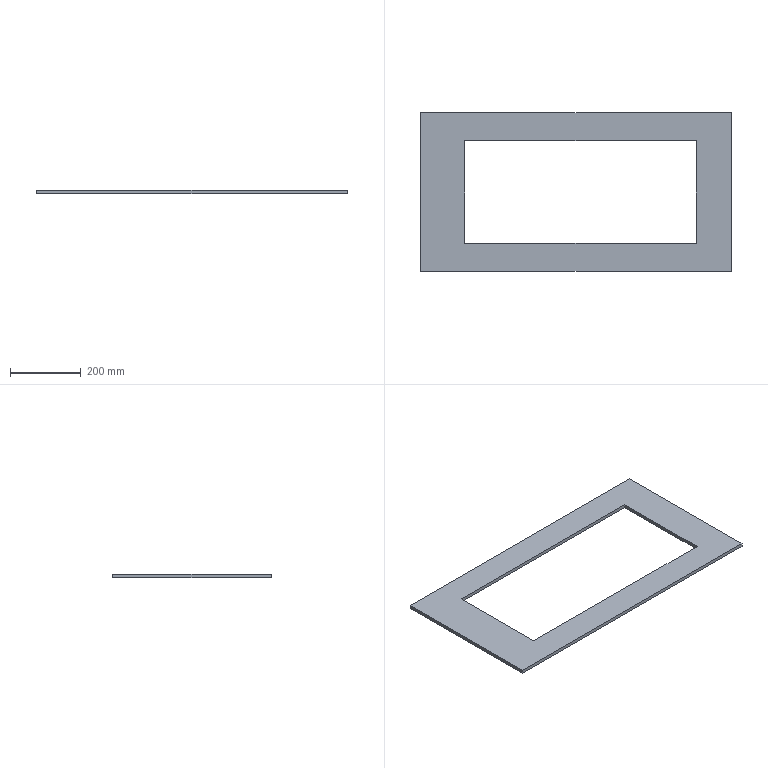Part | STEP file | ceban | 1 solid | 10 faces | box 880 x 450 x 10 mm | volume 2061950 mm3 | plane 10
STEP:
#1=CARTESIAN_POINT('',(0.,0.,0.));
#2=DIRECTION('',(0.,0.,1.));
#3=DIRECTION('',(1.,0.,0.));
#4=AXIS2_PLACEMENT_3D('',#1,#2,#3);
#5=CARTESIAN_POINT('',(440.,-225.,-5.));
#6=VERTEX_POINT('',#5);
#7=CARTESIAN_POINT('',(440.,225.,-5.));
#8=VERTEX_POINT('',#7);
#9=CARTESIAN_POINT('',(440.,225.,-5.));
#10=DIRECTION('',(0.,1.,0.));
#11=VECTOR('',#10,1.);
#12=LINE('',#9,#11);
#13=CARTESIAN_POINT('',(440.,225.,5.));
#14=DIRECTION('',(-1.,0.,0.));
#15=DIRECTION('',(0.,0.,1.));
#16=AXIS2_PLACEMENT_3D('',#13,#14,#15);
#17=PLANE('',#16);
#18=CARTESIAN_POINT('',(-10.,0.));
#19=DIRECTION('',(0.,1.));
#20=VECTOR('',#19,1.);
#21=LINE('',#18,#20);
#22=(GEOMETRIC_REPRESENTATION_CONTEXT(2)PARAMETRIC_REPRESENTATION_CONTEXT()REPRESENTATION_CONTEXT('',''));
#23=DEFINITIONAL_REPRESENTATION('',(#21),#22);
#24=PCURVE('',#17,#23);
#25=CARTESIAN_POINT('',(0.,0.,-5.));
#26=DIRECTION('',(0.,0.,1.));
#27=DIRECTION('',(1.,0.,0.));
#28=AXIS2_PLACEMENT_3D('',#25,#26,#27);
#29=PLANE('',#28);
#30=CARTESIAN_POINT('',(440.,225.));
#31=DIRECTION('',(0.,1.));
#32=VECTOR('',#31,1.);
#33=LINE('',#30,#32);
#34=(GEOMETRIC_REPRESENTATION_CONTEXT(2)PARAMETRIC_REPRESENTATION_CONTEXT()REPRESENTATION_CONTEXT('',''));
#35=DEFINITIONAL_REPRESENTATION('',(#33),#34);
#36=PCURVE('',#29,#35);
#37=SURFACE_CURVE('',#12,(#24,#36),.PCURVE_S1.);
#38=EDGE_CURVE('',#6,#8,#37,.T.);
#39=ORIENTED_EDGE('',*,*,#38,.T.);
#40=CARTESIAN_POINT('',(440.,225.,5.));
#41=VERTEX_POINT('',#40);
#42=CARTESIAN_POINT('',(440.,225.,5.));
#43=DIRECTION('',(0.,0.,-1.));
#44=VECTOR('',#43,1.);
#45=LINE('',#42,#44);
#46=CARTESIAN_POINT('',(0.,0.));
#47=DIRECTION('',(-1.,0.));
#48=VECTOR('',#47,1.);
#49=LINE('',#46,#48);
#50=(GEOMETRIC_REPRESENTATION_CONTEXT(2)PARAMETRIC_REPRESENTATION_CONTEXT()REPRESENTATION_CONTEXT('',''));
#51=DEFINITIONAL_REPRESENTATION('',(#49),#50);
#52=PCURVE('',#17,#51);
#53=CARTESIAN_POINT('',(-440.,225.,5.));
#54=DIRECTION('',(0.,-1.,0.));
#55=DIRECTION('',(0.,0.,-1.));
#56=AXIS2_PLACEMENT_3D('',#53,#54,#55);
#57=PLANE('',#56);
#58=CARTESIAN_POINT('',(0.,880.));
#59=DIRECTION('',(1.,0.));
#60=VECTOR('',#59,1.);
#61=LINE('',#58,#60);
#62=(GEOMETRIC_REPRESENTATION_CONTEXT(2)PARAMETRIC_REPRESENTATION_CONTEXT()REPRESENTATION_CONTEXT('',''));
#63=DEFINITIONAL_REPRESENTATION('',(#61),#62);
#64=PCURVE('',#57,#63);
#65=SURFACE_CURVE('',#45,(#52,#64),.PCURVE_S1.);
#66=EDGE_CURVE('',#41,#8,#65,.T.);
#67=ORIENTED_EDGE('',*,*,#66,.F.);
#68=CARTESIAN_POINT('',(440.,-225.,5.));
#69=VERTEX_POINT('',#68);
#70=CARTESIAN_POINT('',(440.,225.,5.));
#71=DIRECTION('',(0.,1.,0.));
#72=VECTOR('',#71,1.);
#73=LINE('',#70,#72);
#74=CARTESIAN_POINT('',(0.,0.));
#75=DIRECTION('',(0.,1.));
#76=VECTOR('',#75,1.);
#77=LINE('',#74,#76);
#78=(GEOMETRIC_REPRESENTATION_CONTEXT(2)PARAMETRIC_REPRESENTATION_CONTEXT()REPRESENTATION_CONTEXT('',''));
#79=DEFINITIONAL_REPRESENTATION('',(#77),#78);
#80=PCURVE('',#17,#79);
#81=CARTESIAN_POINT('',(0.,0.,5.));
#82=DIRECTION('',(0.,0.,1.));
#83=DIRECTION('',(1.,0.,0.));
#84=AXIS2_PLACEMENT_3D('',#81,#82,#83);
#85=PLANE('',#84);
#86=CARTESIAN_POINT('',(440.,225.));
#87=DIRECTION('',(0.,1.));
#88=VECTOR('',#87,1.);
#89=LINE('',#86,#88);
#90=(GEOMETRIC_REPRESENTATION_CONTEXT(2)PARAMETRIC_REPRESENTATION_CONTEXT()REPRESENTATION_CONTEXT('',''));
#91=DEFINITIONAL_REPRESENTATION('',(#89),#90);
#92=PCURVE('',#85,#91);
#93=SURFACE_CURVE('',#73,(#80,#92),.PCURVE_S1.);
#94=EDGE_CURVE('',#69,#41,#93,.T.);
#95=ORIENTED_EDGE('',*,*,#94,.F.);
#96=CARTESIAN_POINT('',(440.,-225.,5.));
#97=DIRECTION('',(0.,0.,-1.));
#98=VECTOR('',#97,1.);
#99=LINE('',#96,#98);
#100=CARTESIAN_POINT('',(0.,-450.));
#101=DIRECTION('',(-1.,0.));
#102=VECTOR('',#101,1.);
#103=LINE('',#100,#102);
#104=(GEOMETRIC_REPRESENTATION_CONTEXT(2)PARAMETRIC_REPRESENTATION_CONTEXT()REPRESENTATION_CONTEXT('',''));
#105=DEFINITIONAL_REPRESENTATION('',(#103),#104);
#106=PCURVE('',#17,#105);
#107=CARTESIAN_POINT('',(-440.,-225.,5.));
#108=DIRECTION('',(0.,1.,0.));
#109=DIRECTION('',(0.,0.,1.));
#110=AXIS2_PLACEMENT_3D('',#107,#108,#109);
#111=PLANE('',#110);
#112=CARTESIAN_POINT('',(0.,880.));
#113=DIRECTION('',(-1.,0.));
#114=VECTOR('',#113,1.);
#115=LINE('',#112,#114);
#116=(GEOMETRIC_REPRESENTATION_CONTEXT(2)PARAMETRIC_REPRESENTATION_CONTEXT()REPRESENTATION_CONTEXT('',''));
#117=DEFINITIONAL_REPRESENTATION('',(#115),#116);
#118=PCURVE('',#111,#117);
#119=SURFACE_CURVE('',#99,(#106,#118),.PCURVE_S1.);
#120=EDGE_CURVE('',#69,#6,#119,.T.);
#121=ORIENTED_EDGE('',*,*,#120,.T.);
#122=EDGE_LOOP('',(#39,#67,#95,#121));
#123=FACE_BOUND('',#122,.T.);
#124=ADVANCED_FACE('',(#123),#17,.F.);
#125=CARTESIAN_POINT('',(-440.,225.,-5.));
#126=VERTEX_POINT('',#125);
#127=CARTESIAN_POINT('',(-440.,225.,-5.));
#128=DIRECTION('',(-1.,0.,0.));
#129=VECTOR('',#128,1.);
#130=LINE('',#127,#129);
#131=CARTESIAN_POINT('',(10.,0.));
#132=DIRECTION('',(0.,-1.));
#133=VECTOR('',#132,1.);
#134=LINE('',#131,#133);
#135=(GEOMETRIC_REPRESENTATION_CONTEXT(2)PARAMETRIC_REPRESENTATION_CONTEXT()REPRESENTATION_CONTEXT('',''));
#136=DEFINITIONAL_REPRESENTATION('',(#134),#135);
#137=PCURVE('',#57,#136);
#138=CARTESIAN_POINT('',(-440.,225.));
#139=DIRECTION('',(-1.,0.));
#140=VECTOR('',#139,1.);
#141=LINE('',#138,#140);
#142=(GEOMETRIC_REPRESENTATION_CONTEXT(2)PARAMETRIC_REPRESENTATION_CONTEXT()REPRESENTATION_CONTEXT('',''));
#143=DEFINITIONAL_REPRESENTATION('',(#141),#142);
#144=PCURVE('',#29,#143);
#145=SURFACE_CURVE('',#130,(#137,#144),.PCURVE_S1.);
#146=EDGE_CURVE('',#8,#126,#145,.T.);
#147=ORIENTED_EDGE('',*,*,#146,.T.);
#148=CARTESIAN_POINT('',(-440.,225.,5.));
#149=VERTEX_POINT('',#148);
#150=CARTESIAN_POINT('',(-440.,225.,5.));
#151=DIRECTION('',(0.,0.,-1.));
#152=VECTOR('',#151,1.);
#153=LINE('',#150,#152);
#154=CARTESIAN_POINT('',(0.,0.));
#155=DIRECTION('',(1.,0.));
#156=VECTOR('',#155,1.);
#157=LINE('',#154,#156);
#158=(GEOMETRIC_REPRESENTATION_CONTEXT(2)PARAMETRIC_REPRESENTATION_CONTEXT()REPRESENTATION_CONTEXT('',''));
#159=DEFINITIONAL_REPRESENTATION('',(#157),#158);
#160=PCURVE('',#57,#159);
#161=CARTESIAN_POINT('',(-440.,225.,5.));
#162=DIRECTION('',(1.,0.,0.));
#163=DIRECTION('',(0.,1.,0.));
#164=AXIS2_PLACEMENT_3D('',#161,#162,#163);
#165=PLANE('',#164);
#166=CARTESIAN_POINT('',(0.,0.));
#167=DIRECTION('',(0.,-1.));
#168=VECTOR('',#167,1.);
#169=LINE('',#166,#168);
#170=(GEOMETRIC_REPRESENTATION_CONTEXT(2)PARAMETRIC_REPRESENTATION_CONTEXT()REPRESENTATION_CONTEXT('',''));
#171=DEFINITIONAL_REPRESENTATION('',(#169),#170);
#172=PCURVE('',#165,#171);
#173=SURFACE_CURVE('',#153,(#160,#172),.PCURVE_S1.);
#174=EDGE_CURVE('',#149,#126,#173,.T.);
#175=ORIENTED_EDGE('',*,*,#174,.F.);
#176=CARTESIAN_POINT('',(-440.,225.,5.));
#177=DIRECTION('',(-1.,0.,0.));
#178=VECTOR('',#177,1.);
#179=LINE('',#176,#178);
#180=CARTESIAN_POINT('',(0.,0.));
#181=DIRECTION('',(0.,-1.));
#182=VECTOR('',#181,1.);
#183=LINE('',#180,#182);
#184=(GEOMETRIC_REPRESENTATION_CONTEXT(2)PARAMETRIC_REPRESENTATION_CONTEXT()REPRESENTATION_CONTEXT('',''));
#185=DEFINITIONAL_REPRESENTATION('',(#183),#184);
#186=PCURVE('',#57,#185);
#187=CARTESIAN_POINT('',(-440.,225.));
#188=DIRECTION('',(-1.,0.));
#189=VECTOR('',#188,1.);
#190=LINE('',#187,#189);
#191=(GEOMETRIC_REPRESENTATION_CONTEXT(2)PARAMETRIC_REPRESENTATION_CONTEXT()REPRESENTATION_CONTEXT('',''));
#192=DEFINITIONAL_REPRESENTATION('',(#190),#191);
#193=PCURVE('',#85,#192);
#194=SURFACE_CURVE('',#179,(#186,#193),.PCURVE_S1.);
#195=EDGE_CURVE('',#41,#149,#194,.T.);
#196=ORIENTED_EDGE('',*,*,#195,.F.);
#197=ORIENTED_EDGE('',*,*,#66,.T.);
#198=EDGE_LOOP('',(#147,#175,#196,#197));
#199=FACE_BOUND('',#198,.T.);
#200=ADVANCED_FACE('',(#199),#57,.F.);
#201=CARTESIAN_POINT('',(-440.,-225.,-5.));
#202=VERTEX_POINT('',#201);
#203=CARTESIAN_POINT('',(-440.,225.,-5.));
#204=DIRECTION('',(0.,-1.,0.));
#205=VECTOR('',#204,1.);
#206=LINE('',#203,#205);
#207=CARTESIAN_POINT('',(0.,-10.));
#208=DIRECTION('',(-1.,0.));
#209=VECTOR('',#208,1.);
#210=LINE('',#207,#209);
#211=(GEOMETRIC_REPRESENTATION_CONTEXT(2)PARAMETRIC_REPRESENTATION_CONTEXT()REPRESENTATION_CONTEXT('',''));
#212=DEFINITIONAL_REPRESENTATION('',(#210),#211);
#213=PCURVE('',#165,#212);
#214=CARTESIAN_POINT('',(-440.,225.));
#215=DIRECTION('',(0.,-1.));
#216=VECTOR('',#215,1.);
#217=LINE('',#214,#216);
#218=(GEOMETRIC_REPRESENTATION_CONTEXT(2)PARAMETRIC_REPRESENTATION_CONTEXT()REPRESENTATION_CONTEXT('',''));
#219=DEFINITIONAL_REPRESENTATION('',(#217),#218);
#220=PCURVE('',#29,#219);
#221=SURFACE_CURVE('',#206,(#213,#220),.PCURVE_S1.);
#222=EDGE_CURVE('',#126,#202,#221,.T.);
#223=ORIENTED_EDGE('',*,*,#222,.T.);
#224=CARTESIAN_POINT('',(-440.,-225.,5.));
#225=VERTEX_POINT('',#224);
#226=CARTESIAN_POINT('',(-440.,-225.,5.));
#227=DIRECTION('',(0.,0.,-1.));
#228=VECTOR('',#227,1.);
#229=LINE('',#226,#228);
#230=CARTESIAN_POINT('',(-450.,0.));
#231=DIRECTION('',(0.,-1.));
#232=VECTOR('',#231,1.);
#233=LINE('',#230,#232);
#234=(GEOMETRIC_REPRESENTATION_CONTEXT(2)PARAMETRIC_REPRESENTATION_CONTEXT()REPRESENTATION_CONTEXT('',''));
#235=DEFINITIONAL_REPRESENTATION('',(#233),#234);
#236=PCURVE('',#165,#235);
#237=CARTESIAN_POINT('',(0.,0.));
#238=DIRECTION('',(-1.,0.));
#239=VECTOR('',#238,1.);
#240=LINE('',#237,#239);
#241=(GEOMETRIC_REPRESENTATION_CONTEXT(2)PARAMETRIC_REPRESENTATION_CONTEXT()REPRESENTATION_CONTEXT('',''));
#242=DEFINITIONAL_REPRESENTATION('',(#240),#241);
#243=PCURVE('',#111,#242);
#244=SURFACE_CURVE('',#229,(#236,#243),.PCURVE_S1.);
#245=EDGE_CURVE('',#225,#202,#244,.T.);
#246=ORIENTED_EDGE('',*,*,#245,.F.);
#247=CARTESIAN_POINT('',(-440.,225.,5.));
#248=DIRECTION('',(0.,-1.,0.));
#249=VECTOR('',#248,1.);
#250=LINE('',#247,#249);
#251=CARTESIAN_POINT('',(0.,0.));
#252=DIRECTION('',(-1.,0.));
#253=VECTOR('',#252,1.);
#254=LINE('',#251,#253);
#255=(GEOMETRIC_REPRESENTATION_CONTEXT(2)PARAMETRIC_REPRESENTATION_CONTEXT()REPRESENTATION_CONTEXT('',''));
#256=DEFINITIONAL_REPRESENTATION('',(#254),#255);
#257=PCURVE('',#165,#256);
#258=CARTESIAN_POINT('',(-440.,225.));
#259=DIRECTION('',(0.,-1.));
#260=VECTOR('',#259,1.);
#261=LINE('',#258,#260);
#262=(GEOMETRIC_REPRESENTATION_CONTEXT(2)PARAMETRIC_REPRESENTATION_CONTEXT()REPRESENTATION_CONTEXT('',''));
#263=DEFINITIONAL_REPRESENTATION('',(#261),#262);
#264=PCURVE('',#85,#263);
#265=SURFACE_CURVE('',#250,(#257,#264),.PCURVE_S1.);
#266=EDGE_CURVE('',#149,#225,#265,.T.);
#267=ORIENTED_EDGE('',*,*,#266,.F.);
#268=ORIENTED_EDGE('',*,*,#174,.T.);
#269=EDGE_LOOP('',(#223,#246,#267,#268));
#270=FACE_BOUND('',#269,.T.);
#271=ADVANCED_FACE('',(#270),#165,.F.);
#272=CARTESIAN_POINT('',(-440.,-225.,-5.));
#273=DIRECTION('',(1.,0.,0.));
#274=VECTOR('',#273,1.);
#275=LINE('',#272,#274);
#276=CARTESIAN_POINT('',(-10.,0.));
#277=DIRECTION('',(0.,1.));
#278=VECTOR('',#277,1.);
#279=LINE('',#276,#278);
#280=(GEOMETRIC_REPRESENTATION_CONTEXT(2)PARAMETRIC_REPRESENTATION_CONTEXT()REPRESENTATION_CONTEXT('',''));
#281=DEFINITIONAL_REPRESENTATION('',(#279),#280);
#282=PCURVE('',#111,#281);
#283=CARTESIAN_POINT('',(-440.,-225.));
#284=DIRECTION('',(1.,0.));
#285=VECTOR('',#284,1.);
#286=LINE('',#283,#285);
#287=(GEOMETRIC_REPRESENTATION_CONTEXT(2)PARAMETRIC_REPRESENTATION_CONTEXT()REPRESENTATION_CONTEXT('',''));
#288=DEFINITIONAL_REPRESENTATION('',(#286),#287);
#289=PCURVE('',#29,#288);
#290=SURFACE_CURVE('',#275,(#282,#289),.PCURVE_S1.);
#291=EDGE_CURVE('',#202,#6,#290,.T.);
#292=ORIENTED_EDGE('',*,*,#291,.T.);
#293=ORIENTED_EDGE('',*,*,#120,.F.);
#294=CARTESIAN_POINT('',(-440.,-225.,5.));
#295=DIRECTION('',(1.,0.,0.));
#296=VECTOR('',#295,1.);
#297=LINE('',#294,#296);
#298=CARTESIAN_POINT('',(0.,0.));
#299=DIRECTION('',(0.,1.));
#300=VECTOR('',#299,1.);
#301=LINE('',#298,#300);
#302=(GEOMETRIC_REPRESENTATION_CONTEXT(2)PARAMETRIC_REPRESENTATION_CONTEXT()REPRESENTATION_CONTEXT('',''));
#303=DEFINITIONAL_REPRESENTATION('',(#301),#302);
#304=PCURVE('',#111,#303);
#305=CARTESIAN_POINT('',(-440.,-225.));
#306=DIRECTION('',(1.,0.));
#307=VECTOR('',#306,1.);
#308=LINE('',#305,#307);
#309=(GEOMETRIC_REPRESENTATION_CONTEXT(2)PARAMETRIC_REPRESENTATION_CONTEXT()REPRESENTATION_CONTEXT('',''));
#310=DEFINITIONAL_REPRESENTATION('',(#308),#309);
#311=PCURVE('',#85,#310);
#312=SURFACE_CURVE('',#297,(#304,#311),.PCURVE_S1.);
#313=EDGE_CURVE('',#225,#69,#312,.T.);
#314=ORIENTED_EDGE('',*,*,#313,.F.);
#315=ORIENTED_EDGE('',*,*,#245,.T.);
#316=EDGE_LOOP('',(#292,#293,#314,#315));
#317=FACE_BOUND('',#316,.T.);
#318=ADVANCED_FACE('',(#317),#111,.F.);
#319=CARTESIAN_POINT('',(-314.5,145.,5.));
#320=VERTEX_POINT('',#319);
#321=CARTESIAN_POINT('',(-314.5,-145.,5.));
#322=VERTEX_POINT('',#321);
#323=CARTESIAN_POINT('',(-314.5,145.,5.));
#324=DIRECTION('',(0.,-1.,0.));
#325=VECTOR('',#324,1.);
#326=LINE('',#323,#325);
#327=CARTESIAN_POINT('',(-314.5,145.));
#328=DIRECTION('',(0.,-1.));
#329=VECTOR('',#328,1.);
#330=LINE('',#327,#329);
#331=(GEOMETRIC_REPRESENTATION_CONTEXT(2)PARAMETRIC_REPRESENTATION_CONTEXT()REPRESENTATION_CONTEXT('',''));
#332=DEFINITIONAL_REPRESENTATION('',(#330),#331);
#333=PCURVE('',#85,#332);
#334=CARTESIAN_POINT('',(-314.5,145.,-5.));
#335=DIRECTION('',(-1.,0.,0.));
#336=DIRECTION('',(0.,0.,1.));
#337=AXIS2_PLACEMENT_3D('',#334,#335,#336);
#338=PLANE('',#337);
#339=CARTESIAN_POINT('',(10.,0.));
#340=DIRECTION('',(0.,-1.));
#341=VECTOR('',#340,1.);
#342=LINE('',#339,#341);
#343=(GEOMETRIC_REPRESENTATION_CONTEXT(2)PARAMETRIC_REPRESENTATION_CONTEXT()REPRESENTATION_CONTEXT('',''));
#344=DEFINITIONAL_REPRESENTATION('',(#342),#343);
#345=PCURVE('',#338,#344);
#346=SURFACE_CURVE('',#326,(#333,#345),.PCURVE_S1.);
#347=EDGE_CURVE('',#320,#322,#346,.T.);
#348=ORIENTED_EDGE('',*,*,#347,.F.);
#349=CARTESIAN_POINT('',(340.,145.,5.));
#350=VERTEX_POINT('',#349);
#351=CARTESIAN_POINT('',(-314.5,145.,5.));
#352=DIRECTION('',(-1.,0.,0.));
#353=VECTOR('',#352,1.);
#354=LINE('',#351,#353);
#355=CARTESIAN_POINT('',(-314.5,145.));
#356=DIRECTION('',(-1.,0.));
#357=VECTOR('',#356,1.);
#358=LINE('',#355,#357);
#359=(GEOMETRIC_REPRESENTATION_CONTEXT(2)PARAMETRIC_REPRESENTATION_CONTEXT()REPRESENTATION_CONTEXT('',''));
#360=DEFINITIONAL_REPRESENTATION('',(#358),#359);
#361=PCURVE('',#85,#360);
#362=CARTESIAN_POINT('',(-314.5,145.,-5.));
#363=DIRECTION('',(0.,1.,0.));
#364=DIRECTION('',(0.,0.,1.));
#365=AXIS2_PLACEMENT_3D('',#362,#363,#364);
#366=PLANE('',#365);
#367=CARTESIAN_POINT('',(10.,0.));
#368=DIRECTION('',(0.,-1.));
#369=VECTOR('',#368,1.);
#370=LINE('',#367,#369);
#371=(GEOMETRIC_REPRESENTATION_CONTEXT(2)PARAMETRIC_REPRESENTATION_CONTEXT()REPRESENTATION_CONTEXT('',''));
#372=DEFINITIONAL_REPRESENTATION('',(#370),#371);
#373=PCURVE('',#366,#372);
#374=SURFACE_CURVE('',#354,(#361,#373),.PCURVE_S1.);
#375=EDGE_CURVE('',#350,#320,#374,.T.);
#376=ORIENTED_EDGE('',*,*,#375,.F.);
#377=CARTESIAN_POINT('',(340.,-145.,5.));
#378=VERTEX_POINT('',#377);
#379=CARTESIAN_POINT('',(340.,145.,5.));
#380=DIRECTION('',(0.,1.,0.));
#381=VECTOR('',#380,1.);
#382=LINE('',#379,#381);
#383=CARTESIAN_POINT('',(340.,145.));
#384=DIRECTION('',(0.,1.));
#385=VECTOR('',#384,1.);
#386=LINE('',#383,#385);
#387=(GEOMETRIC_REPRESENTATION_CONTEXT(2)PARAMETRIC_REPRESENTATION_CONTEXT()REPRESENTATION_CONTEXT('',''));
#388=DEFINITIONAL_REPRESENTATION('',(#386),#387);
#389=PCURVE('',#85,#388);
#390=CARTESIAN_POINT('',(340.,145.,-5.));
#391=DIRECTION('',(1.,0.,0.));
#392=DIRECTION('',(0.,1.,0.));
#393=AXIS2_PLACEMENT_3D('',#390,#391,#392);
#394=PLANE('',#393);
#395=CARTESIAN_POINT('',(0.,10.));
#396=DIRECTION('',(1.,0.));
#397=VECTOR('',#396,1.);
#398=LINE('',#395,#397);
#399=(GEOMETRIC_REPRESENTATION_CONTEXT(2)PARAMETRIC_REPRESENTATION_CONTEXT()REPRESENTATION_CONTEXT('',''));
#400=DEFINITIONAL_REPRESENTATION('',(#398),#399);
#401=PCURVE('',#394,#400);
#402=SURFACE_CURVE('',#382,(#389,#401),.PCURVE_S1.);
#403=EDGE_CURVE('',#378,#350,#402,.T.);
#404=ORIENTED_EDGE('',*,*,#403,.F.);
#405=CARTESIAN_POINT('',(-314.5,-145.,5.));
#406=DIRECTION('',(1.,0.,0.));
#407=VECTOR('',#406,1.);
#408=LINE('',#405,#407);
#409=CARTESIAN_POINT('',(-314.5,-145.));
#410=DIRECTION('',(1.,0.));
#411=VECTOR('',#410,1.);
#412=LINE('',#409,#411);
#413=(GEOMETRIC_REPRESENTATION_CONTEXT(2)PARAMETRIC_REPRESENTATION_CONTEXT()REPRESENTATION_CONTEXT('',''));
#414=DEFINITIONAL_REPRESENTATION('',(#412),#413);
#415=PCURVE('',#85,#414);
#416=CARTESIAN_POINT('',(-314.5,-145.,-5.));
#417=DIRECTION('',(0.,-1.,0.));
#418=DIRECTION('',(0.,0.,-1.));
#419=AXIS2_PLACEMENT_3D('',#416,#417,#418);
#420=PLANE('',#419);
#421=CARTESIAN_POINT('',(-10.,0.));
#422=DIRECTION('',(0.,1.));
#423=VECTOR('',#422,1.);
#424=LINE('',#421,#423);
#425=(GEOMETRIC_REPRESENTATION_CONTEXT(2)PARAMETRIC_REPRESENTATION_CONTEXT()REPRESENTATION_CONTEXT('',''));
#426=DEFINITIONAL_REPRESENTATION('',(#424),#425);
#427=PCURVE('',#420,#426);
#428=SURFACE_CURVE('',#408,(#415,#427),.PCURVE_S1.);
#429=EDGE_CURVE('',#322,#378,#428,.T.);
#430=ORIENTED_EDGE('',*,*,#429,.F.);
#431=EDGE_LOOP('',(#348,#376,#404,#430));
#432=FACE_BOUND('',#431,.T.);
#433=ORIENTED_EDGE('',*,*,#94,.T.);
#434=ORIENTED_EDGE('',*,*,#195,.T.);
#435=ORIENTED_EDGE('',*,*,#266,.T.);
#436=ORIENTED_EDGE('',*,*,#313,.T.);
#437=EDGE_LOOP('',(#433,#434,#435,#436));
#438=FACE_BOUND('',#437,.T.);
#439=ADVANCED_FACE('',(#432,#438),#85,.T.);
#440=CARTESIAN_POINT('',(340.,145.,-5.));
#441=VERTEX_POINT('',#440);
#442=CARTESIAN_POINT('',(-314.5,145.,-5.));
#443=VERTEX_POINT('',#442);
#444=CARTESIAN_POINT('',(-314.5,145.,-5.));
#445=DIRECTION('',(-1.,0.,0.));
#446=VECTOR('',#445,1.);
#447=LINE('',#444,#446);
#448=CARTESIAN_POINT('',(-314.5,145.));
#449=DIRECTION('',(-1.,0.));
#450=VECTOR('',#449,1.);
#451=LINE('',#448,#450);
#452=(GEOMETRIC_REPRESENTATION_CONTEXT(2)PARAMETRIC_REPRESENTATION_CONTEXT()REPRESENTATION_CONTEXT('',''));
#453=DEFINITIONAL_REPRESENTATION('',(#451),#452);
#454=PCURVE('',#29,#453);
#455=CARTESIAN_POINT('',(0.,0.));
#456=DIRECTION('',(0.,-1.));
#457=VECTOR('',#456,1.);
#458=LINE('',#455,#457);
#459=(GEOMETRIC_REPRESENTATION_CONTEXT(2)PARAMETRIC_REPRESENTATION_CONTEXT()REPRESENTATION_CONTEXT('',''));
#460=DEFINITIONAL_REPRESENTATION('',(#458),#459);
#461=PCURVE('',#366,#460);
#462=SURFACE_CURVE('',#447,(#454,#461),.PCURVE_S1.);
#463=EDGE_CURVE('',#441,#443,#462,.T.);
#464=ORIENTED_EDGE('',*,*,#463,.T.);
#465=CARTESIAN_POINT('',(-314.5,-145.,-5.));
#466=VERTEX_POINT('',#465);
#467=CARTESIAN_POINT('',(-314.5,145.,-5.));
#468=DIRECTION('',(0.,-1.,0.));
#469=VECTOR('',#468,1.);
#470=LINE('',#467,#469);
#471=CARTESIAN_POINT('',(-314.5,145.));
#472=DIRECTION('',(0.,-1.));
#473=VECTOR('',#472,1.);
#474=LINE('',#471,#473);
#475=(GEOMETRIC_REPRESENTATION_CONTEXT(2)PARAMETRIC_REPRESENTATION_CONTEXT()REPRESENTATION_CONTEXT('',''));
#476=DEFINITIONAL_REPRESENTATION('',(#474),#475);
#477=PCURVE('',#29,#476);
#478=CARTESIAN_POINT('',(0.,0.));
#479=DIRECTION('',(0.,-1.));
#480=VECTOR('',#479,1.);
#481=LINE('',#478,#480);
#482=(GEOMETRIC_REPRESENTATION_CONTEXT(2)PARAMETRIC_REPRESENTATION_CONTEXT()REPRESENTATION_CONTEXT('',''));
#483=DEFINITIONAL_REPRESENTATION('',(#481),#482);
#484=PCURVE('',#338,#483);
#485=SURFACE_CURVE('',#470,(#477,#484),.PCURVE_S1.);
#486=EDGE_CURVE('',#443,#466,#485,.T.);
#487=ORIENTED_EDGE('',*,*,#486,.T.);
#488=CARTESIAN_POINT('',(340.,-145.,-5.));
#489=VERTEX_POINT('',#488);
#490=CARTESIAN_POINT('',(-314.5,-145.,-5.));
#491=DIRECTION('',(1.,0.,0.));
#492=VECTOR('',#491,1.);
#493=LINE('',#490,#492);
#494=CARTESIAN_POINT('',(-314.5,-145.));
#495=DIRECTION('',(1.,0.));
#496=VECTOR('',#495,1.);
#497=LINE('',#494,#496);
#498=(GEOMETRIC_REPRESENTATION_CONTEXT(2)PARAMETRIC_REPRESENTATION_CONTEXT()REPRESENTATION_CONTEXT('',''));
#499=DEFINITIONAL_REPRESENTATION('',(#497),#498);
#500=PCURVE('',#29,#499);
#501=CARTESIAN_POINT('',(0.,0.));
#502=DIRECTION('',(0.,1.));
#503=VECTOR('',#502,1.);
#504=LINE('',#501,#503);
#505=(GEOMETRIC_REPRESENTATION_CONTEXT(2)PARAMETRIC_REPRESENTATION_CONTEXT()REPRESENTATION_CONTEXT('',''));
#506=DEFINITIONAL_REPRESENTATION('',(#504),#505);
#507=PCURVE('',#420,#506);
#508=SURFACE_CURVE('',#493,(#500,#507),.PCURVE_S1.);
#509=EDGE_CURVE('',#466,#489,#508,.T.);
#510=ORIENTED_EDGE('',*,*,#509,.T.);
#511=CARTESIAN_POINT('',(340.,145.,-5.));
#512=DIRECTION('',(0.,1.,0.));
#513=VECTOR('',#512,1.);
#514=LINE('',#511,#513);
#515=CARTESIAN_POINT('',(340.,145.));
#516=DIRECTION('',(0.,1.));
#517=VECTOR('',#516,1.);
#518=LINE('',#515,#517);
#519=(GEOMETRIC_REPRESENTATION_CONTEXT(2)PARAMETRIC_REPRESENTATION_CONTEXT()REPRESENTATION_CONTEXT('',''));
#520=DEFINITIONAL_REPRESENTATION('',(#518),#519);
#521=PCURVE('',#29,#520);
#522=CARTESIAN_POINT('',(0.,0.));
#523=DIRECTION('',(1.,0.));
#524=VECTOR('',#523,1.);
#525=LINE('',#522,#524);
#526=(GEOMETRIC_REPRESENTATION_CONTEXT(2)PARAMETRIC_REPRESENTATION_CONTEXT()REPRESENTATION_CONTEXT('',''));
#527=DEFINITIONAL_REPRESENTATION('',(#525),#526);
#528=PCURVE('',#394,#527);
#529=SURFACE_CURVE('',#514,(#521,#528),.PCURVE_S1.);
#530=EDGE_CURVE('',#489,#441,#529,.T.);
#531=ORIENTED_EDGE('',*,*,#530,.T.);
#532=EDGE_LOOP('',(#464,#487,#510,#531));
#533=FACE_BOUND('',#532,.T.);
#534=ORIENTED_EDGE('',*,*,#38,.F.);
#535=ORIENTED_EDGE('',*,*,#291,.F.);
#536=ORIENTED_EDGE('',*,*,#222,.F.);
#537=ORIENTED_EDGE('',*,*,#146,.F.);
#538=EDGE_LOOP('',(#534,#535,#536,#537));
#539=FACE_BOUND('',#538,.T.);
#540=ADVANCED_FACE('',(#533,#539),#29,.F.);
#541=ORIENTED_EDGE('',*,*,#347,.T.);
#542=CARTESIAN_POINT('',(-314.5,-145.,-5.));
#543=DIRECTION('',(0.,0.,1.));
#544=VECTOR('',#543,1.);
#545=LINE('',#542,#544);
#546=CARTESIAN_POINT('',(0.,-290.));
#547=DIRECTION('',(1.,0.));
#548=VECTOR('',#547,1.);
#549=LINE('',#546,#548);
#550=(GEOMETRIC_REPRESENTATION_CONTEXT(2)PARAMETRIC_REPRESENTATION_CONTEXT()REPRESENTATION_CONTEXT('',''));
#551=DEFINITIONAL_REPRESENTATION('',(#549),#550);
#552=PCURVE('',#338,#551);
#553=CARTESIAN_POINT('',(0.,0.));
#554=DIRECTION('',(-1.,0.));
#555=VECTOR('',#554,1.);
#556=LINE('',#553,#555);
#557=(GEOMETRIC_REPRESENTATION_CONTEXT(2)PARAMETRIC_REPRESENTATION_CONTEXT()REPRESENTATION_CONTEXT('',''));
#558=DEFINITIONAL_REPRESENTATION('',(#556),#557);
#559=PCURVE('',#420,#558);
#560=SURFACE_CURVE('',#545,(#552,#559),.PCURVE_S1.);
#561=EDGE_CURVE('',#466,#322,#560,.T.);
#562=ORIENTED_EDGE('',*,*,#561,.F.);
#563=ORIENTED_EDGE('',*,*,#486,.F.);
#564=CARTESIAN_POINT('',(-314.5,145.,-5.));
#565=DIRECTION('',(0.,0.,1.));
#566=VECTOR('',#565,1.);
#567=LINE('',#564,#566);
#568=CARTESIAN_POINT('',(0.,0.));
#569=DIRECTION('',(1.,0.));
#570=VECTOR('',#569,1.);
#571=LINE('',#568,#570);
#572=(GEOMETRIC_REPRESENTATION_CONTEXT(2)PARAMETRIC_REPRESENTATION_CONTEXT()REPRESENTATION_CONTEXT('',''));
#573=DEFINITIONAL_REPRESENTATION('',(#571),#572);
#574=PCURVE('',#338,#573);
#575=CARTESIAN_POINT('',(0.,0.));
#576=DIRECTION('',(1.,0.));
#577=VECTOR('',#576,1.);
#578=LINE('',#575,#577);
#579=(GEOMETRIC_REPRESENTATION_CONTEXT(2)PARAMETRIC_REPRESENTATION_CONTEXT()REPRESENTATION_CONTEXT('',''));
#580=DEFINITIONAL_REPRESENTATION('',(#578),#579);
#581=PCURVE('',#366,#580);
#582=SURFACE_CURVE('',#567,(#574,#581),.PCURVE_S1.);
#583=EDGE_CURVE('',#443,#320,#582,.T.);
#584=ORIENTED_EDGE('',*,*,#583,.T.);
#585=EDGE_LOOP('',(#541,#562,#563,#584));
#586=FACE_BOUND('',#585,.T.);
#587=ADVANCED_FACE('',(#586),#338,.F.);
#588=ORIENTED_EDGE('',*,*,#375,.T.);
#589=ORIENTED_EDGE('',*,*,#583,.F.);
#590=ORIENTED_EDGE('',*,*,#463,.F.);
#591=CARTESIAN_POINT('',(340.,145.,-5.));
#592=DIRECTION('',(0.,0.,1.));
#593=VECTOR('',#592,1.);
#594=LINE('',#591,#593);
#595=CARTESIAN_POINT('',(0.,654.5));
#596=DIRECTION('',(1.,0.));
#597=VECTOR('',#596,1.);
#598=LINE('',#595,#597);
#599=(GEOMETRIC_REPRESENTATION_CONTEXT(2)PARAMETRIC_REPRESENTATION_CONTEXT()REPRESENTATION_CONTEXT('',''));
#600=DEFINITIONAL_REPRESENTATION('',(#598),#599);
#601=PCURVE('',#366,#600);
#602=CARTESIAN_POINT('',(0.,0.));
#603=DIRECTION('',(0.,1.));
#604=VECTOR('',#603,1.);
#605=LINE('',#602,#604);
#606=(GEOMETRIC_REPRESENTATION_CONTEXT(2)PARAMETRIC_REPRESENTATION_CONTEXT()REPRESENTATION_CONTEXT('',''));
#607=DEFINITIONAL_REPRESENTATION('',(#605),#606);
#608=PCURVE('',#394,#607);
#609=SURFACE_CURVE('',#594,(#601,#608),.PCURVE_S1.);
#610=EDGE_CURVE('',#441,#350,#609,.T.);
#611=ORIENTED_EDGE('',*,*,#610,.T.);
#612=EDGE_LOOP('',(#588,#589,#590,#611));
#613=FACE_BOUND('',#612,.T.);
#614=ADVANCED_FACE('',(#613),#366,.F.);
#615=ORIENTED_EDGE('',*,*,#403,.T.);
#616=ORIENTED_EDGE('',*,*,#610,.F.);
#617=ORIENTED_EDGE('',*,*,#530,.F.);
#618=CARTESIAN_POINT('',(340.,-145.,-5.));
#619=DIRECTION('',(0.,0.,1.));
#620=VECTOR('',#619,1.);
#621=LINE('',#618,#620);
#622=CARTESIAN_POINT('',(-290.,0.));
#623=DIRECTION('',(0.,1.));
#624=VECTOR('',#623,1.);
#625=LINE('',#622,#624);
#626=(GEOMETRIC_REPRESENTATION_CONTEXT(2)PARAMETRIC_REPRESENTATION_CONTEXT()REPRESENTATION_CONTEXT('',''));
#627=DEFINITIONAL_REPRESENTATION('',(#625),#626);
#628=PCURVE('',#394,#627);
#629=CARTESIAN_POINT('',(0.,654.5));
#630=DIRECTION('',(-1.,0.));
#631=VECTOR('',#630,1.);
#632=LINE('',#629,#631);
#633=(GEOMETRIC_REPRESENTATION_CONTEXT(2)PARAMETRIC_REPRESENTATION_CONTEXT()REPRESENTATION_CONTEXT('',''));
#634=DEFINITIONAL_REPRESENTATION('',(#632),#633);
#635=PCURVE('',#420,#634);
#636=SURFACE_CURVE('',#621,(#628,#635),.PCURVE_S1.);
#637=EDGE_CURVE('',#489,#378,#636,.T.);
#638=ORIENTED_EDGE('',*,*,#637,.T.);
#639=EDGE_LOOP('',(#615,#616,#617,#638));
#640=FACE_BOUND('',#639,.T.);
#641=ADVANCED_FACE('',(#640),#394,.F.);
#642=ORIENTED_EDGE('',*,*,#429,.T.);
#643=ORIENTED_EDGE('',*,*,#637,.F.);
#644=ORIENTED_EDGE('',*,*,#509,.F.);
#645=ORIENTED_EDGE('',*,*,#561,.T.);
#646=EDGE_LOOP('',(#642,#643,#644,#645));
#647=FACE_BOUND('',#646,.T.);
#648=ADVANCED_FACE('',(#647),#420,.F.);
#649=CLOSED_SHELL('',(#124,#200,#271,#318,#439,#540,#587,#614,#641,#648));
#650=MANIFOLD_SOLID_BREP('',#649);
#651=(LENGTH_UNIT()NAMED_UNIT(*)SI_UNIT(.MILLI.,.METRE.));
#652=UNCERTAINTY_MEASURE_WITH_UNIT(LENGTH_MEASURE(0.0000001),#651,'','');
#653=(NAMED_UNIT(*)PLANE_ANGLE_UNIT()SI_UNIT($,.RADIAN.));
#654=(NAMED_UNIT(*)SI_UNIT($,.STERADIAN.)SOLID_ANGLE_UNIT());
#655=(GEOMETRIC_REPRESENTATION_CONTEXT(3)GLOBAL_UNCERTAINTY_ASSIGNED_CONTEXT((#652))GLOBAL_UNIT_ASSIGNED_CONTEXT((#651,#653,#654))REPRESENTATION_CONTEXT('',''));
#656=ADVANCED_BREP_SHAPE_REPRESENTATION('',(#4,#650),#655);